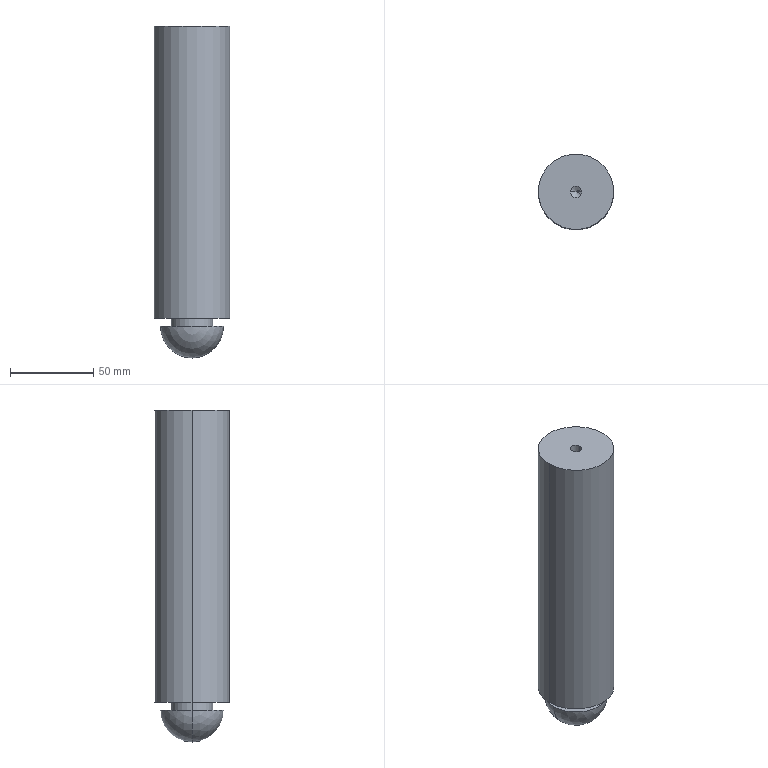Part | SolidWorks | features 3DProfileFeature 1, HoleWzd 1, SavedExtBody 1 | 1 solid | 13 faces | box 45.5 x 45.5 x 200 mm | volume 302158 mm3 | cylinder 6 | plane 3 | cone 2 | sphere 2 | commonest cylinder face diameters 6.8 x2 25 x2 45.5 x2
STEP:
#1=CARTESIAN_POINT('',(-3.4,0.,-22.25));
#2=VERTEX_POINT('',#1);
#3=CARTESIAN_POINT('',(3.4,0.,-22.25));
#4=VERTEX_POINT('',#3);
#5=CARTESIAN_POINT('',(0.,0.,-22.25));
#6=DIRECTION('',(0.,0.,1.));
#7=DIRECTION('',(1.,0.,0.));
#8=AXIS2_PLACEMENT_3D('',#5,#6,#7);
#9=CIRCLE('',#8,3.4);
#10=EDGE_CURVE('',#2,#4,#9,.T.);
#11=ORIENTED_EDGE('',*,*,#10,.F.);
#12=CARTESIAN_POINT('',(-3.4,0.,0.));
#13=VERTEX_POINT('',#12);
#14=CARTESIAN_POINT('',(-3.4,0.,0.));
#15=DIRECTION('',(0.,0.,1.));
#16=VECTOR('',#15,1000.);
#17=LINE('',#14,#16);
#18=EDGE_CURVE('',#2,#13,#17,.T.);
#19=ORIENTED_EDGE('',*,*,#18,.T.);
#20=CARTESIAN_POINT('',(3.4,0.,0.));
#21=VERTEX_POINT('',#20);
#22=CARTESIAN_POINT('',(0.,0.,0.));
#23=DIRECTION('',(0.,0.,1.));
#24=DIRECTION('',(1.,0.,0.));
#25=AXIS2_PLACEMENT_3D('',#22,#23,#24);
#26=CIRCLE('',#25,3.4);
#27=EDGE_CURVE('',#13,#21,#26,.T.);
#28=ORIENTED_EDGE('',*,*,#27,.T.);
#29=CARTESIAN_POINT('',(3.4,0.,0.));
#30=DIRECTION('',(0.,0.,1.));
#31=VECTOR('',#30,1000.);
#32=LINE('',#29,#31);
#33=EDGE_CURVE('',#4,#21,#32,.T.);
#34=ORIENTED_EDGE('',*,*,#33,.F.);
#35=EDGE_LOOP('',(#11,#19,#28,#34));
#36=FACE_OUTER_BOUND('',#35,.T.);
#37=CARTESIAN_POINT('',(0.,0.,0.));
#38=DIRECTION('',(0.,0.,1.));
#39=DIRECTION('',(1.,0.,0.));
#40=AXIS2_PLACEMENT_3D('',#37,#38,#39);
#41=CYLINDRICAL_SURFACE('',#40,3.4);
#42=ADVANCED_FACE('',(#36),#41,.F.);
#43=CARTESIAN_POINT('',(0.,0.,-24.293));
#44=VERTEX_POINT('',#43);
#45=CARTESIAN_POINT('',(3.4,0.,-22.25));
#46=DIRECTION('',(0.8572,0.,0.515));
#47=VECTOR('',#46,1000.);
#48=LINE('',#45,#47);
#49=EDGE_CURVE('',#44,#4,#48,.T.);
#50=ORIENTED_EDGE('',*,*,#49,.F.);
#51=CARTESIAN_POINT('',(-3.4,0.,-22.25));
#52=DIRECTION('',(-0.8572,0.,0.515));
#53=VECTOR('',#52,1000.);
#54=LINE('',#51,#53);
#55=EDGE_CURVE('',#44,#2,#54,.T.);
#56=ORIENTED_EDGE('',*,*,#55,.T.);
#57=ORIENTED_EDGE('',*,*,#10,.T.);
#58=EDGE_LOOP('',(#50,#56,#57));
#59=FACE_OUTER_BOUND('',#58,.T.);
#60=CARTESIAN_POINT('',(0.,0.,-22.25));
#61=DIRECTION('',(0.,0.,1.));
#62=DIRECTION('',(1.,0.,0.));
#63=AXIS2_PLACEMENT_3D('',#60,#61,#62);
#64=CONICAL_SURFACE('',#63,3.4,1.03);
#65=ADVANCED_FACE('',(#59),#64,.F.);
#66=CARTESIAN_POINT('',(-19.,0.,-181.));
#67=VERTEX_POINT('',#66);
#68=CARTESIAN_POINT('',(19.,0.,-181.));
#69=VERTEX_POINT('',#68);
#70=CARTESIAN_POINT('',(0.,0.,-181.));
#71=DIRECTION('',(0.,0.,1.));
#72=DIRECTION('',(-1.,0.,0.));
#73=AXIS2_PLACEMENT_3D('',#70,#71,#72);
#74=CIRCLE('',#73,19.);
#75=EDGE_CURVE('',#67,#69,#74,.T.);
#76=ORIENTED_EDGE('',*,*,#75,.F.);
#77=CARTESIAN_POINT('',(0.,0.,-200.));
#78=VERTEX_POINT('',#77);
#79=CARTESIAN_POINT('',(0.,0.,-181.));
#80=DIRECTION('',(0.,-1.,0.));
#81=DIRECTION('',(1.,0.,0.));
#82=AXIS2_PLACEMENT_3D('',#79,#80,#81);
#83=CIRCLE('',#82,19.);
#84=EDGE_CURVE('',#67,#78,#83,.T.);
#85=ORIENTED_EDGE('',*,*,#84,.T.);
#86=CARTESIAN_POINT('',(0.,0.,-181.));
#87=DIRECTION('',(0.,1.,0.));
#88=DIRECTION('',(0.,0.,1.));
#89=AXIS2_PLACEMENT_3D('',#86,#87,#88);
#90=CIRCLE('',#89,19.);
#91=EDGE_CURVE('',#69,#78,#90,.T.);
#92=ORIENTED_EDGE('',*,*,#91,.F.);
#93=EDGE_LOOP('',(#76,#85,#92));
#94=FACE_OUTER_BOUND('',#93,.T.);
#95=CARTESIAN_POINT('',(0.,0.,-181.));
#96=DIRECTION('',(0.,-1.,0.));
#97=DIRECTION('',(1.,0.,0.));
#98=AXIS2_PLACEMENT_3D('',#95,#96,#97);
#99=SPHERICAL_SURFACE('',#98,19.);
#100=ADVANCED_FACE('',(#94),#99,.T.);
#101=CARTESIAN_POINT('',(-12.5,0.,-176.));
#102=VERTEX_POINT('',#101);
#103=CARTESIAN_POINT('',(12.5,0.,-176.));
#104=VERTEX_POINT('',#103);
#105=CARTESIAN_POINT('',(0.,0.,-176.));
#106=DIRECTION('',(0.,0.,-1.));
#107=DIRECTION('',(-1.,0.,0.));
#108=AXIS2_PLACEMENT_3D('',#105,#106,#107);
#109=CIRCLE('',#108,12.5);
#110=EDGE_CURVE('',#102,#104,#109,.T.);
#111=ORIENTED_EDGE('',*,*,#110,.T.);
#112=CARTESIAN_POINT('',(12.5,0.,-181.));
#113=VERTEX_POINT('',#112);
#114=CARTESIAN_POINT('',(12.5,0.,-188.));
#115=DIRECTION('',(0.,0.,-1.));
#116=VECTOR('',#115,1000.);
#117=LINE('',#114,#116);
#118=EDGE_CURVE('',#104,#113,#117,.T.);
#119=ORIENTED_EDGE('',*,*,#118,.T.);
#120=CARTESIAN_POINT('',(-12.5,0.,-181.));
#121=VERTEX_POINT('',#120);
#122=CARTESIAN_POINT('',(0.,0.,-181.));
#123=DIRECTION('',(0.,0.,-1.));
#124=DIRECTION('',(-1.,0.,0.));
#125=AXIS2_PLACEMENT_3D('',#122,#123,#124);
#126=CIRCLE('',#125,12.5);
#127=EDGE_CURVE('',#121,#113,#126,.T.);
#128=ORIENTED_EDGE('',*,*,#127,.F.);
#129=CARTESIAN_POINT('',(-12.5,0.,-188.));
#130=DIRECTION('',(0.,0.,-1.));
#131=VECTOR('',#130,1000.);
#132=LINE('',#129,#131);
#133=EDGE_CURVE('',#102,#121,#132,.T.);
#134=ORIENTED_EDGE('',*,*,#133,.F.);
#135=EDGE_LOOP('',(#111,#119,#128,#134));
#136=FACE_OUTER_BOUND('',#135,.T.);
#137=CARTESIAN_POINT('',(0.,0.,-188.));
#138=DIRECTION('',(0.,0.,-1.));
#139=DIRECTION('',(-1.,0.,0.));
#140=AXIS2_PLACEMENT_3D('',#137,#138,#139);
#141=CYLINDRICAL_SURFACE('',#140,12.5);
#142=ADVANCED_FACE('',(#136),#141,.T.);
#143=CARTESIAN_POINT('',(-22.75,0.,-176.));
#144=VERTEX_POINT('',#143);
#145=CARTESIAN_POINT('',(22.75,0.,-176.));
#146=VERTEX_POINT('',#145);
#147=CARTESIAN_POINT('',(0.,0.,-176.));
#148=DIRECTION('',(0.,0.,-1.));
#149=DIRECTION('',(-1.,0.,0.));
#150=AXIS2_PLACEMENT_3D('',#147,#148,#149);
#151=CIRCLE('',#150,22.75);
#152=EDGE_CURVE('',#144,#146,#151,.T.);
#153=ORIENTED_EDGE('',*,*,#152,.F.);
#154=CARTESIAN_POINT('',(-22.75,0.,0.));
#155=VERTEX_POINT('',#154);
#156=CARTESIAN_POINT('',(-22.75,0.,-200.));
#157=DIRECTION('',(0.,0.,1.));
#158=VECTOR('',#157,1000.);
#159=LINE('',#156,#158);
#160=EDGE_CURVE('',#144,#155,#159,.T.);
#161=ORIENTED_EDGE('',*,*,#160,.T.);
#162=CARTESIAN_POINT('',(22.75,0.,0.));
#163=VERTEX_POINT('',#162);
#164=CARTESIAN_POINT('',(0.,0.,0.));
#165=DIRECTION('',(0.,0.,-1.));
#166=DIRECTION('',(-1.,0.,0.));
#167=AXIS2_PLACEMENT_3D('',#164,#165,#166);
#168=CIRCLE('',#167,22.75);
#169=EDGE_CURVE('',#155,#163,#168,.T.);
#170=ORIENTED_EDGE('',*,*,#169,.T.);
#171=CARTESIAN_POINT('',(22.75,0.,-200.));
#172=DIRECTION('',(0.,0.,1.));
#173=VECTOR('',#172,1000.);
#174=LINE('',#171,#173);
#175=EDGE_CURVE('',#146,#163,#174,.T.);
#176=ORIENTED_EDGE('',*,*,#175,.F.);
#177=EDGE_LOOP('',(#153,#161,#170,#176));
#178=FACE_OUTER_BOUND('',#177,.T.);
#179=CARTESIAN_POINT('',(0.,0.,-200.));
#180=DIRECTION('',(0.,0.,1.));
#181=DIRECTION('',(1.,0.,0.));
#182=AXIS2_PLACEMENT_3D('',#179,#180,#181);
#183=CYLINDRICAL_SURFACE('',#182,22.75);
#184=ADVANCED_FACE('',(#178),#183,.T.);
#185=ORIENTED_EDGE('',*,*,#160,.F.);
#186=CARTESIAN_POINT('',(0.,0.,-176.));
#187=DIRECTION('',(0.,0.,-1.));
#188=DIRECTION('',(-1.,0.,0.));
#189=AXIS2_PLACEMENT_3D('',#186,#187,#188);
#190=CIRCLE('',#189,22.75);
#191=EDGE_CURVE('',#146,#144,#190,.T.);
#192=ORIENTED_EDGE('',*,*,#191,.F.);
#193=ORIENTED_EDGE('',*,*,#175,.T.);
#194=CARTESIAN_POINT('',(0.,0.,0.));
#195=DIRECTION('',(0.,0.,-1.));
#196=DIRECTION('',(-1.,0.,0.));
#197=AXIS2_PLACEMENT_3D('',#194,#195,#196);
#198=CIRCLE('',#197,22.75);
#199=EDGE_CURVE('',#163,#155,#198,.T.);
#200=ORIENTED_EDGE('',*,*,#199,.T.);
#201=EDGE_LOOP('',(#185,#192,#193,#200));
#202=FACE_OUTER_BOUND('',#201,.T.);
#203=CARTESIAN_POINT('',(0.,0.,-200.));
#204=DIRECTION('',(0.,0.,1.));
#205=DIRECTION('',(1.,0.,0.));
#206=AXIS2_PLACEMENT_3D('',#203,#204,#205);
#207=CYLINDRICAL_SURFACE('',#206,22.75);
#208=ADVANCED_FACE('',(#202),#207,.T.);
#209=CARTESIAN_POINT('',(0.,0.,0.));
#210=DIRECTION('',(0.,0.,1.));
#211=DIRECTION('',(1.,0.,0.));
#212=AXIS2_PLACEMENT_3D('',#209,#210,#211);
#213=CIRCLE('',#212,3.4);
#214=EDGE_CURVE('',#21,#13,#213,.T.);
#215=ORIENTED_EDGE('',*,*,#214,.F.);
#216=ORIENTED_EDGE('',*,*,#27,.F.);
#217=EDGE_LOOP('',(#215,#216));
#218=FACE_BOUND('',#217,.T.);
#219=ORIENTED_EDGE('',*,*,#199,.F.);
#220=ORIENTED_EDGE('',*,*,#169,.F.);
#221=EDGE_LOOP('',(#219,#220));
#222=FACE_OUTER_BOUND('',#221,.T.);
#223=CARTESIAN_POINT('',(0.,0.,0.));
#224=DIRECTION('',(0.,0.,-1.));
#225=DIRECTION('',(-1.,0.,0.));
#226=AXIS2_PLACEMENT_3D('',#223,#224,#225);
#227=PLANE('',#226);
#228=ADVANCED_FACE('',(#218,#222),#227,.F.);
#229=CARTESIAN_POINT('',(0.,0.,-181.));
#230=DIRECTION('',(0.,0.,1.));
#231=DIRECTION('',(-1.,0.,0.));
#232=AXIS2_PLACEMENT_3D('',#229,#230,#231);
#233=CIRCLE('',#232,19.);
#234=EDGE_CURVE('',#69,#67,#233,.T.);
#235=ORIENTED_EDGE('',*,*,#234,.T.);
#236=ORIENTED_EDGE('',*,*,#75,.T.);
#237=EDGE_LOOP('',(#235,#236));
#238=FACE_OUTER_BOUND('',#237,.T.);
#239=ORIENTED_EDGE('',*,*,#127,.T.);
#240=CARTESIAN_POINT('',(0.,0.,-181.));
#241=DIRECTION('',(0.,0.,-1.));
#242=DIRECTION('',(-1.,0.,0.));
#243=AXIS2_PLACEMENT_3D('',#240,#241,#242);
#244=CIRCLE('',#243,12.5);
#245=EDGE_CURVE('',#113,#121,#244,.T.);
#246=ORIENTED_EDGE('',*,*,#245,.T.);
#247=EDGE_LOOP('',(#239,#246));
#248=FACE_BOUND('',#247,.T.);
#249=CARTESIAN_POINT('',(-22.75,0.,-181.));
#250=DIRECTION('',(0.,0.,-1.));
#251=DIRECTION('',(-1.,0.,0.));
#252=AXIS2_PLACEMENT_3D('',#249,#250,#251);
#253=PLANE('',#252);
#254=ADVANCED_FACE('',(#238,#248),#253,.F.);
#255=ORIENTED_EDGE('',*,*,#118,.F.);
#256=CARTESIAN_POINT('',(0.,0.,-176.));
#257=DIRECTION('',(0.,0.,-1.));
#258=DIRECTION('',(-1.,0.,0.));
#259=AXIS2_PLACEMENT_3D('',#256,#257,#258);
#260=CIRCLE('',#259,12.5);
#261=EDGE_CURVE('',#104,#102,#260,.T.);
#262=ORIENTED_EDGE('',*,*,#261,.T.);
#263=ORIENTED_EDGE('',*,*,#133,.T.);
#264=ORIENTED_EDGE('',*,*,#245,.F.);
#265=EDGE_LOOP('',(#255,#262,#263,#264));
#266=FACE_OUTER_BOUND('',#265,.T.);
#267=CARTESIAN_POINT('',(0.,0.,-188.));
#268=DIRECTION('',(0.,0.,-1.));
#269=DIRECTION('',(-1.,0.,0.));
#270=AXIS2_PLACEMENT_3D('',#267,#268,#269);
#271=CYLINDRICAL_SURFACE('',#270,12.5);
#272=ADVANCED_FACE('',(#266),#271,.T.);
#273=ORIENTED_EDGE('',*,*,#110,.F.);
#274=ORIENTED_EDGE('',*,*,#261,.F.);
#275=EDGE_LOOP('',(#273,#274));
#276=FACE_BOUND('',#275,.T.);
#277=ORIENTED_EDGE('',*,*,#191,.T.);
#278=ORIENTED_EDGE('',*,*,#152,.T.);
#279=EDGE_LOOP('',(#277,#278));
#280=FACE_OUTER_BOUND('',#279,.T.);
#281=CARTESIAN_POINT('',(-22.75,0.,-176.));
#282=DIRECTION('',(0.,0.,1.));
#283=DIRECTION('',(1.,0.,0.));
#284=AXIS2_PLACEMENT_3D('',#281,#282,#283);
#285=PLANE('',#284);
#286=ADVANCED_FACE('',(#276,#280),#285,.F.);
#287=ORIENTED_EDGE('',*,*,#84,.F.);
#288=ORIENTED_EDGE('',*,*,#234,.F.);
#289=ORIENTED_EDGE('',*,*,#91,.T.);
#290=EDGE_LOOP('',(#287,#288,#289));
#291=FACE_OUTER_BOUND('',#290,.T.);
#292=CARTESIAN_POINT('',(0.,0.,-181.));
#293=DIRECTION('',(0.,-1.,0.));
#294=DIRECTION('',(1.,0.,0.));
#295=AXIS2_PLACEMENT_3D('',#292,#293,#294);
#296=SPHERICAL_SURFACE('',#295,19.);
#297=ADVANCED_FACE('',(#291),#296,.T.);
#298=ORIENTED_EDGE('',*,*,#55,.F.);
#299=ORIENTED_EDGE('',*,*,#49,.T.);
#300=CARTESIAN_POINT('',(0.,0.,-22.25));
#301=DIRECTION('',(0.,0.,1.));
#302=DIRECTION('',(1.,0.,0.));
#303=AXIS2_PLACEMENT_3D('',#300,#301,#302);
#304=CIRCLE('',#303,3.4);
#305=EDGE_CURVE('',#4,#2,#304,.T.);
#306=ORIENTED_EDGE('',*,*,#305,.T.);
#307=EDGE_LOOP('',(#298,#299,#306));
#308=FACE_OUTER_BOUND('',#307,.T.);
#309=CARTESIAN_POINT('',(0.,0.,-22.25));
#310=DIRECTION('',(0.,0.,1.));
#311=DIRECTION('',(1.,0.,0.));
#312=AXIS2_PLACEMENT_3D('',#309,#310,#311);
#313=CONICAL_SURFACE('',#312,3.4,1.03);
#314=ADVANCED_FACE('',(#308),#313,.F.);
#315=ORIENTED_EDGE('',*,*,#18,.F.);
#316=ORIENTED_EDGE('',*,*,#305,.F.);
#317=ORIENTED_EDGE('',*,*,#33,.T.);
#318=ORIENTED_EDGE('',*,*,#214,.T.);
#319=EDGE_LOOP('',(#315,#316,#317,#318));
#320=FACE_OUTER_BOUND('',#319,.T.);
#321=CARTESIAN_POINT('',(0.,0.,0.));
#322=DIRECTION('',(0.,0.,1.));
#323=DIRECTION('',(1.,0.,0.));
#324=AXIS2_PLACEMENT_3D('',#321,#322,#323);
#325=CYLINDRICAL_SURFACE('',#324,3.4);
#326=ADVANCED_FACE('',(#320),#325,.F.);
#327=CLOSED_SHELL('',(#42,#65,#100,#142,#184,#208,#228,#254,#272,#286,#297,#314,#326));
#328=MANIFOLD_SOLID_BREP('',#327);
#329=CARTESIAN_POINT('',(0.,0.,0.));
#330=DIRECTION('',(0.,0.,1.));
#331=DIRECTION('',(1.,0.,0.));
#332=AXIS2_PLACEMENT_3D('',#329,#330,#331);
#333=(LENGTH_UNIT()NAMED_UNIT(*)SI_UNIT(.MILLI.,.METRE.));
#334=UNCERTAINTY_MEASURE_WITH_UNIT(LENGTH_MEASURE(0.00001),#333,'','');
#335=(NAMED_UNIT(*)PLANE_ANGLE_UNIT()SI_UNIT($,.RADIAN.));
#336=(NAMED_UNIT(*)SI_UNIT($,.STERADIAN.)SOLID_ANGLE_UNIT());
#337=(GEOMETRIC_REPRESENTATION_CONTEXT(3)GLOBAL_UNCERTAINTY_ASSIGNED_CONTEXT((#334))GLOBAL_UNIT_ASSIGNED_CONTEXT((#333,#335,#336))REPRESENTATION_CONTEXT('',''));
#338=ADVANCED_BREP_SHAPE_REPRESENTATION('',(#328,#332),#337);